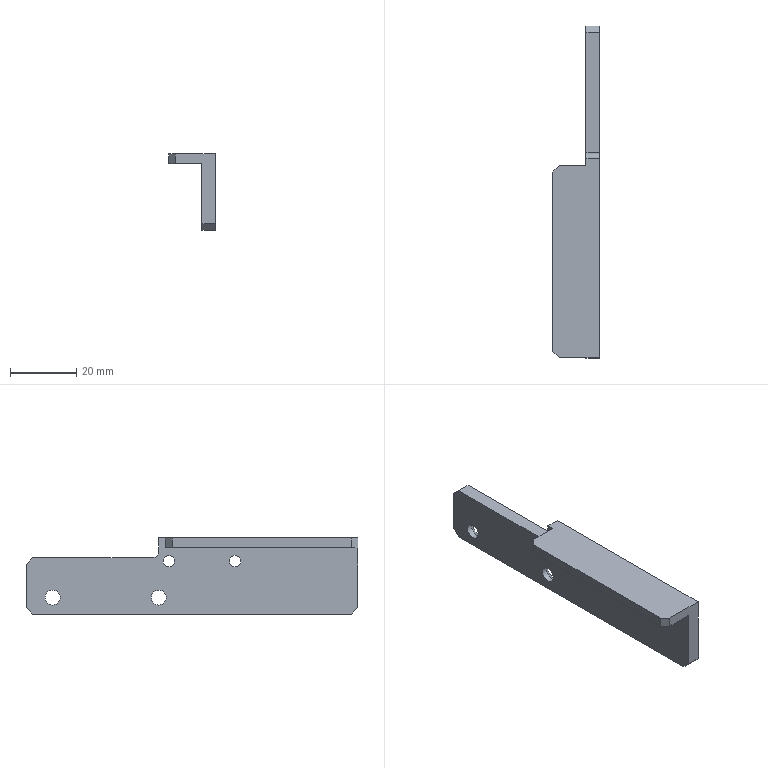Part | NX | features BREP 1 | 1 solid | 25 faces | box 14 x 100 x 23 mm | volume 9598 mm3 | plane 16 | cylinder 5 | cone 4 | commonest cylinder face diameters 3.4 x2 4.5 x2 4 x1
STEP:
#1=CARTESIAN_POINT('',(7.,50.,3.5));
#2=VERTEX_POINT('',#1);
#3=CARTESIAN_POINT('',(7.,50.,-9.5));
#4=VERTEX_POINT('',#3);
#5=CARTESIAN_POINT('',(7.,50.,11.5));
#6=DIRECTION('',(0.,0.,-1.));
#7=VECTOR('',#6,1000.);
#8=LINE('',#5,#7);
#9=EDGE_CURVE('',#2,#4,#8,.T.);
#10=ORIENTED_EDGE('',*,*,#9,.T.);
#11=CARTESIAN_POINT('',(3.,50.,-9.5));
#12=VERTEX_POINT('',#11);
#13=CARTESIAN_POINT('',(3.,50.,-9.5));
#14=DIRECTION('',(-1.,0.,0.));
#15=VECTOR('',#14,1000.);
#16=LINE('',#13,#15);
#17=EDGE_CURVE('',#4,#12,#16,.T.);
#18=ORIENTED_EDGE('',*,*,#17,.T.);
#19=CARTESIAN_POINT('',(3.,50.,3.5));
#20=VERTEX_POINT('',#19);
#21=CARTESIAN_POINT('',(3.,50.,-11.5));
#22=DIRECTION('',(0.,0.,-1.));
#23=VECTOR('',#22,1000.);
#24=LINE('',#21,#23);
#25=EDGE_CURVE('',#20,#12,#24,.T.);
#26=ORIENTED_EDGE('',*,*,#25,.F.);
#27=CARTESIAN_POINT('',(7.,50.,3.5));
#28=DIRECTION('',(1.,0.,0.));
#29=VECTOR('',#28,1000.);
#30=LINE('',#27,#29);
#31=EDGE_CURVE('',#20,#2,#30,.T.);
#32=ORIENTED_EDGE('',*,*,#31,.T.);
#33=EDGE_LOOP('',(#10,#18,#26,#32));
#34=FACE_BOUND('',#33,.T.);
#35=CARTESIAN_POINT('',(-7.,50.,11.5));
#36=DIRECTION('',(0.,-1.,0.));
#37=DIRECTION('',(0.,0.,1.));
#38=AXIS2_PLACEMENT_3D('',#35,#36,#37);
#39=PLANE('',#38);
#40=ADVANCED_FACE('',(#34),#39,.F.);
#41=CARTESIAN_POINT('',(7.,7.,1.03));
#42=VERTEX_POINT('',#41);
#43=CARTESIAN_POINT('',(7.,7.,4.5));
#44=DIRECTION('',(1.,0.,0.));
#45=DIRECTION('',(0.,0.,-1.));
#46=AXIS2_PLACEMENT_3D('',#43,#44,#45);
#47=CIRCLE('',#46,3.47);
#48=EDGE_CURVE('',#42,#42,#47,.T.);
#49=ORIENTED_EDGE('',*,*,#48,.F.);
#50=EDGE_LOOP('',(#49));
#51=FACE_BOUND('',#50,.T.);
#52=CARTESIAN_POINT('',(7.,-13.,1.03));
#53=VERTEX_POINT('',#52);
#54=CARTESIAN_POINT('',(7.,-13.,4.5));
#55=DIRECTION('',(1.,0.,0.));
#56=DIRECTION('',(0.,0.,-1.));
#57=AXIS2_PLACEMENT_3D('',#54,#55,#56);
#58=CIRCLE('',#57,3.47);
#59=EDGE_CURVE('',#53,#53,#58,.T.);
#60=ORIENTED_EDGE('',*,*,#59,.F.);
#61=EDGE_LOOP('',(#60));
#62=FACE_BOUND('',#61,.T.);
#63=CARTESIAN_POINT('',(7.,42.,-11.09));
#64=VERTEX_POINT('',#63);
#65=CARTESIAN_POINT('',(7.,42.,-6.5));
#66=DIRECTION('',(1.,0.,0.));
#67=DIRECTION('',(0.,0.,-1.));
#68=AXIS2_PLACEMENT_3D('',#65,#66,#67);
#69=CIRCLE('',#68,4.59);
#70=EDGE_CURVE('',#64,#64,#69,.T.);
#71=ORIENTED_EDGE('',*,*,#70,.F.);
#72=EDGE_LOOP('',(#71));
#73=FACE_BOUND('',#72,.T.);
#74=CARTESIAN_POINT('',(7.,10.,-11.09));
#75=VERTEX_POINT('',#74);
#76=CARTESIAN_POINT('',(7.,10.,-6.5));
#77=DIRECTION('',(1.,0.,0.));
#78=DIRECTION('',(0.,0.,-1.));
#79=AXIS2_PLACEMENT_3D('',#76,#77,#78);
#80=CIRCLE('',#79,4.59);
#81=EDGE_CURVE('',#75,#75,#80,.T.);
#82=ORIENTED_EDGE('',*,*,#81,.F.);
#83=EDGE_LOOP('',(#82));
#84=FACE_BOUND('',#83,.T.);
#85=CARTESIAN_POINT('',(7.,-50.,11.5));
#86=VERTEX_POINT('',#85);
#87=CARTESIAN_POINT('',(7.,-50.,-9.5));
#88=VERTEX_POINT('',#87);
#89=CARTESIAN_POINT('',(7.,-50.,11.5));
#90=DIRECTION('',(0.,0.,-1.));
#91=VECTOR('',#90,1000.);
#92=LINE('',#89,#91);
#93=EDGE_CURVE('',#86,#88,#92,.T.);
#94=ORIENTED_EDGE('',*,*,#93,.T.);
#95=CARTESIAN_POINT('',(7.,-48.,-11.5));
#96=VERTEX_POINT('',#95);
#97=CARTESIAN_POINT('',(7.,-50.,-9.5));
#98=DIRECTION('',(0.,0.7071,-0.7071));
#99=VECTOR('',#98,1000.);
#100=LINE('',#97,#99);
#101=EDGE_CURVE('',#88,#96,#100,.T.);
#102=ORIENTED_EDGE('',*,*,#101,.T.);
#103=CARTESIAN_POINT('',(7.,48.,-11.5));
#104=VERTEX_POINT('',#103);
#105=CARTESIAN_POINT('',(7.,-50.,-11.5));
#106=DIRECTION('',(0.,1.,0.));
#107=VECTOR('',#106,1000.);
#108=LINE('',#105,#107);
#109=EDGE_CURVE('',#96,#104,#108,.T.);
#110=ORIENTED_EDGE('',*,*,#109,.T.);
#111=CARTESIAN_POINT('',(7.,50.,-9.5));
#112=DIRECTION('',(0.,0.7071,0.7071));
#113=VECTOR('',#112,1000.);
#114=LINE('',#111,#113);
#115=EDGE_CURVE('',#104,#4,#114,.T.);
#116=ORIENTED_EDGE('',*,*,#115,.T.);
#117=ORIENTED_EDGE('',*,*,#9,.F.);
#118=CARTESIAN_POINT('',(7.,48.,5.5));
#119=VERTEX_POINT('',#118);
#120=CARTESIAN_POINT('',(7.,48.,5.5));
#121=DIRECTION('',(0.,-0.7071,0.7071));
#122=VECTOR('',#121,1000.);
#123=LINE('',#120,#122);
#124=EDGE_CURVE('',#2,#119,#123,.T.);
#125=ORIENTED_EDGE('',*,*,#124,.T.);
#126=CARTESIAN_POINT('',(7.,12.,5.5));
#127=VERTEX_POINT('',#126);
#128=CARTESIAN_POINT('',(7.,50.,5.5));
#129=DIRECTION('',(0.,1.,0.));
#130=VECTOR('',#129,1000.);
#131=LINE('',#128,#130);
#132=EDGE_CURVE('',#127,#119,#131,.T.);
#133=ORIENTED_EDGE('',*,*,#132,.F.);
#134=CARTESIAN_POINT('',(7.,10.,7.5));
#135=VERTEX_POINT('',#134);
#136=CARTESIAN_POINT('',(7.,12.,7.5));
#137=DIRECTION('',(-1.,0.,0.));
#138=DIRECTION('',(0.,0.,1.));
#139=AXIS2_PLACEMENT_3D('',#136,#137,#138);
#140=CIRCLE('',#139,2.);
#141=EDGE_CURVE('',#127,#135,#140,.T.);
#142=ORIENTED_EDGE('',*,*,#141,.T.);
#143=CARTESIAN_POINT('',(7.,10.,11.5));
#144=VERTEX_POINT('',#143);
#145=CARTESIAN_POINT('',(7.,10.,5.5));
#146=DIRECTION('',(0.,0.,1.));
#147=VECTOR('',#146,1000.);
#148=LINE('',#145,#147);
#149=EDGE_CURVE('',#135,#144,#148,.T.);
#150=ORIENTED_EDGE('',*,*,#149,.T.);
#151=CARTESIAN_POINT('',(7.,-50.,11.5));
#152=DIRECTION('',(0.,1.,0.));
#153=VECTOR('',#152,1000.);
#154=LINE('',#151,#153);
#155=EDGE_CURVE('',#86,#144,#154,.T.);
#156=ORIENTED_EDGE('',*,*,#155,.F.);
#157=EDGE_LOOP('',(#94,#102,#110,#116,#117,#125,#133,#142,#150,#156));
#158=FACE_BOUND('',#157,.T.);
#159=CARTESIAN_POINT('',(7.,-50.,11.5));
#160=DIRECTION('',(-1.,0.,0.));
#161=DIRECTION('',(0.,0.,-1.));
#162=AXIS2_PLACEMENT_3D('',#159,#160,#161);
#163=PLANE('',#162);
#164=ADVANCED_FACE('',(#51,#62,#73,#84,#158),#163,.F.);
#165=CARTESIAN_POINT('',(-7.,-48.,8.5));
#166=VERTEX_POINT('',#165);
#167=CARTESIAN_POINT('',(-7.,6.,8.5));
#168=VERTEX_POINT('',#167);
#169=CARTESIAN_POINT('',(-7.,-72.361,8.5));
#170=DIRECTION('',(0.,1.,0.));
#171=VECTOR('',#170,1000.);
#172=LINE('',#169,#171);
#173=EDGE_CURVE('',#166,#168,#172,.T.);
#174=ORIENTED_EDGE('',*,*,#173,.F.);
#175=CARTESIAN_POINT('',(-7.,-48.,11.5));
#176=VERTEX_POINT('',#175);
#177=CARTESIAN_POINT('',(-7.,-48.,11.5));
#178=DIRECTION('',(0.,0.,1.));
#179=VECTOR('',#178,1000.);
#180=LINE('',#177,#179);
#181=EDGE_CURVE('',#166,#176,#180,.T.);
#182=ORIENTED_EDGE('',*,*,#181,.T.);
#183=CARTESIAN_POINT('',(-7.,6.,11.5));
#184=VERTEX_POINT('',#183);
#185=CARTESIAN_POINT('',(-7.,-50.,11.5));
#186=DIRECTION('',(0.,-1.,0.));
#187=VECTOR('',#186,1000.);
#188=LINE('',#185,#187);
#189=EDGE_CURVE('',#184,#176,#188,.T.);
#190=ORIENTED_EDGE('',*,*,#189,.F.);
#191=CARTESIAN_POINT('',(-7.,6.,11.5));
#192=DIRECTION('',(0.,0.,-1.));
#193=VECTOR('',#192,1000.);
#194=LINE('',#191,#193);
#195=EDGE_CURVE('',#184,#168,#194,.T.);
#196=ORIENTED_EDGE('',*,*,#195,.T.);
#197=EDGE_LOOP('',(#174,#182,#190,#196));
#198=FACE_BOUND('',#197,.T.);
#199=CARTESIAN_POINT('',(-7.,-50.,11.5));
#200=DIRECTION('',(1.,0.,0.));
#201=DIRECTION('',(0.,0.,1.));
#202=AXIS2_PLACEMENT_3D('',#199,#200,#201);
#203=PLANE('',#202);
#204=ADVANCED_FACE('',(#198),#203,.F.);
#205=CARTESIAN_POINT('',(3.,-50.,-9.5));
#206=VERTEX_POINT('',#205);
#207=CARTESIAN_POINT('',(3.,-50.,8.5));
#208=VERTEX_POINT('',#207);
#209=CARTESIAN_POINT('',(3.,-50.,-11.5));
#210=DIRECTION('',(0.,0.,1.));
#211=VECTOR('',#210,1000.);
#212=LINE('',#209,#211);
#213=EDGE_CURVE('',#206,#208,#212,.T.);
#214=ORIENTED_EDGE('',*,*,#213,.F.);
#215=CARTESIAN_POINT('',(7.,-50.,-9.5));
#216=DIRECTION('',(1.,0.,0.));
#217=VECTOR('',#216,1000.);
#218=LINE('',#215,#217);
#219=EDGE_CURVE('',#206,#88,#218,.T.);
#220=ORIENTED_EDGE('',*,*,#219,.T.);
#221=ORIENTED_EDGE('',*,*,#93,.F.);
#222=CARTESIAN_POINT('',(-5.,-50.,11.5));
#223=VERTEX_POINT('',#222);
#224=CARTESIAN_POINT('',(-7.,-50.,11.5));
#225=DIRECTION('',(1.,0.,0.));
#226=VECTOR('',#225,1000.);
#227=LINE('',#224,#226);
#228=EDGE_CURVE('',#223,#86,#227,.T.);
#229=ORIENTED_EDGE('',*,*,#228,.F.);
#230=CARTESIAN_POINT('',(-5.,-50.,8.5));
#231=VERTEX_POINT('',#230);
#232=CARTESIAN_POINT('',(-5.,-50.,11.5));
#233=DIRECTION('',(0.,0.,-1.));
#234=VECTOR('',#233,1000.);
#235=LINE('',#232,#234);
#236=EDGE_CURVE('',#223,#231,#235,.T.);
#237=ORIENTED_EDGE('',*,*,#236,.T.);
#238=CARTESIAN_POINT('',(-7.,-50.,8.5));
#239=DIRECTION('',(-1.,0.,0.));
#240=VECTOR('',#239,1000.);
#241=LINE('',#238,#240);
#242=EDGE_CURVE('',#208,#231,#241,.T.);
#243=ORIENTED_EDGE('',*,*,#242,.F.);
#244=EDGE_LOOP('',(#214,#220,#221,#229,#237,#243));
#245=FACE_BOUND('',#244,.T.);
#246=CARTESIAN_POINT('',(-7.,-50.,11.5));
#247=DIRECTION('',(0.,1.,0.));
#248=DIRECTION('',(0.,0.,-1.));
#249=AXIS2_PLACEMENT_3D('',#246,#247,#248);
#250=PLANE('',#249);
#251=ADVANCED_FACE('',(#245),#250,.F.);
#252=ORIENTED_EDGE('',*,*,#189,.T.);
#253=CARTESIAN_POINT('',(-5.,-50.,11.5));
#254=DIRECTION('',(0.7071,-0.7071,0.));
#255=VECTOR('',#254,1000.);
#256=LINE('',#253,#255);
#257=EDGE_CURVE('',#176,#223,#256,.T.);
#258=ORIENTED_EDGE('',*,*,#257,.T.);
#259=ORIENTED_EDGE('',*,*,#228,.T.);
#260=ORIENTED_EDGE('',*,*,#155,.T.);
#261=CARTESIAN_POINT('',(3.,10.,11.5));
#262=VERTEX_POINT('',#261);
#263=CARTESIAN_POINT('',(-7.,10.,11.5));
#264=DIRECTION('',(1.,0.,0.));
#265=VECTOR('',#264,1000.);
#266=LINE('',#263,#265);
#267=EDGE_CURVE('',#262,#144,#266,.T.);
#268=ORIENTED_EDGE('',*,*,#267,.F.);
#269=CARTESIAN_POINT('',(3.,8.,11.5));
#270=VERTEX_POINT('',#269);
#271=CARTESIAN_POINT('',(3.,8.,11.5));
#272=DIRECTION('',(0.,1.,0.));
#273=VECTOR('',#272,1000.);
#274=LINE('',#271,#273);
#275=EDGE_CURVE('',#270,#262,#274,.T.);
#276=ORIENTED_EDGE('',*,*,#275,.F.);
#277=CARTESIAN_POINT('',(-5.,8.,11.5));
#278=VERTEX_POINT('',#277);
#279=CARTESIAN_POINT('',(3.,8.,11.5));
#280=DIRECTION('',(1.,0.,0.));
#281=VECTOR('',#280,1000.);
#282=LINE('',#279,#281);
#283=EDGE_CURVE('',#278,#270,#282,.T.);
#284=ORIENTED_EDGE('',*,*,#283,.F.);
#285=CARTESIAN_POINT('',(-5.,8.,11.5));
#286=DIRECTION('',(-0.7071,-0.7071,0.));
#287=VECTOR('',#286,1000.);
#288=LINE('',#285,#287);
#289=EDGE_CURVE('',#278,#184,#288,.T.);
#290=ORIENTED_EDGE('',*,*,#289,.T.);
#291=EDGE_LOOP('',(#252,#258,#259,#260,#268,#276,#284,#290));
#292=FACE_BOUND('',#291,.T.);
#293=CARTESIAN_POINT('',(0.,0.,11.5));
#294=DIRECTION('',(0.,0.,-1.));
#295=DIRECTION('',(1.,0.,0.));
#296=AXIS2_PLACEMENT_3D('',#293,#294,#295);
#297=PLANE('',#296);
#298=ADVANCED_FACE('',(#292),#297,.F.);
#299=ORIENTED_EDGE('',*,*,#109,.F.);
#300=CARTESIAN_POINT('',(3.,-48.,-11.5));
#301=VERTEX_POINT('',#300);
#302=CARTESIAN_POINT('',(3.,-48.,-11.5));
#303=DIRECTION('',(-1.,0.,0.));
#304=VECTOR('',#303,1000.);
#305=LINE('',#302,#304);
#306=EDGE_CURVE('',#96,#301,#305,.T.);
#307=ORIENTED_EDGE('',*,*,#306,.T.);
#308=CARTESIAN_POINT('',(3.,48.,-11.5));
#309=VERTEX_POINT('',#308);
#310=CARTESIAN_POINT('',(3.,-72.361,-11.5));
#311=DIRECTION('',(0.,1.,0.));
#312=VECTOR('',#311,1000.);
#313=LINE('',#310,#312);
#314=EDGE_CURVE('',#301,#309,#313,.T.);
#315=ORIENTED_EDGE('',*,*,#314,.T.);
#316=CARTESIAN_POINT('',(7.,48.,-11.5));
#317=DIRECTION('',(1.,0.,0.));
#318=VECTOR('',#317,1000.);
#319=LINE('',#316,#318);
#320=EDGE_CURVE('',#309,#104,#319,.T.);
#321=ORIENTED_EDGE('',*,*,#320,.T.);
#322=EDGE_LOOP('',(#299,#307,#315,#321));
#323=FACE_BOUND('',#322,.T.);
#324=CARTESIAN_POINT('',(0.,0.,-11.5));
#325=DIRECTION('',(0.,0.,-1.));
#326=DIRECTION('',(1.,0.,0.));
#327=AXIS2_PLACEMENT_3D('',#324,#325,#326);
#328=PLANE('',#327);
#329=ADVANCED_FACE('',(#323),#328,.T.);
#330=CARTESIAN_POINT('',(3.,7.,2.8));
#331=VERTEX_POINT('',#330);
#332=CARTESIAN_POINT('',(3.,7.,4.5));
#333=DIRECTION('',(1.,0.,0.));
#334=DIRECTION('',(0.,0.,-1.));
#335=AXIS2_PLACEMENT_3D('',#332,#333,#334);
#336=CIRCLE('',#335,1.7);
#337=EDGE_CURVE('',#331,#331,#336,.T.);
#338=ORIENTED_EDGE('',*,*,#337,.T.);
#339=EDGE_LOOP('',(#338));
#340=FACE_BOUND('',#339,.T.);
#341=CARTESIAN_POINT('',(3.,-13.,2.8));
#342=VERTEX_POINT('',#341);
#343=CARTESIAN_POINT('',(3.,-13.,4.5));
#344=DIRECTION('',(1.,0.,0.));
#345=DIRECTION('',(0.,0.,-1.));
#346=AXIS2_PLACEMENT_3D('',#343,#344,#345);
#347=CIRCLE('',#346,1.7);
#348=EDGE_CURVE('',#342,#342,#347,.T.);
#349=ORIENTED_EDGE('',*,*,#348,.T.);
#350=EDGE_LOOP('',(#349));
#351=FACE_BOUND('',#350,.T.);
#352=CARTESIAN_POINT('',(3.,42.,-8.75));
#353=VERTEX_POINT('',#352);
#354=CARTESIAN_POINT('',(3.,42.,-6.5));
#355=DIRECTION('',(1.,0.,0.));
#356=DIRECTION('',(0.,0.,-1.));
#357=AXIS2_PLACEMENT_3D('',#354,#355,#356);
#358=CIRCLE('',#357,2.25);
#359=EDGE_CURVE('',#353,#353,#358,.T.);
#360=ORIENTED_EDGE('',*,*,#359,.T.);
#361=EDGE_LOOP('',(#360));
#362=FACE_BOUND('',#361,.T.);
#363=CARTESIAN_POINT('',(3.,10.,-8.75));
#364=VERTEX_POINT('',#363);
#365=CARTESIAN_POINT('',(3.,10.,-6.5));
#366=DIRECTION('',(1.,0.,0.));
#367=DIRECTION('',(0.,0.,-1.));
#368=AXIS2_PLACEMENT_3D('',#365,#366,#367);
#369=CIRCLE('',#368,2.25);
#370=EDGE_CURVE('',#364,#364,#369,.T.);
#371=ORIENTED_EDGE('',*,*,#370,.T.);
#372=EDGE_LOOP('',(#371));
#373=FACE_BOUND('',#372,.T.);
#374=ORIENTED_EDGE('',*,*,#314,.F.);
#375=CARTESIAN_POINT('',(3.,-50.,-9.5));
#376=DIRECTION('',(0.,-0.7071,0.7071));
#377=VECTOR('',#376,1000.);
#378=LINE('',#375,#377);
#379=EDGE_CURVE('',#301,#206,#378,.T.);
#380=ORIENTED_EDGE('',*,*,#379,.T.);
#381=ORIENTED_EDGE('',*,*,#213,.T.);
#382=CARTESIAN_POINT('',(3.,8.,8.5));
#383=VERTEX_POINT('',#382);
#384=CARTESIAN_POINT('',(3.,-72.361,8.5));
#385=DIRECTION('',(0.,1.,0.));
#386=VECTOR('',#385,1000.);
#387=LINE('',#384,#386);
#388=EDGE_CURVE('',#208,#383,#387,.T.);
#389=ORIENTED_EDGE('',*,*,#388,.T.);
#390=CARTESIAN_POINT('',(3.,8.,8.5));
#391=DIRECTION('',(0.,0.,-1.));
#392=VECTOR('',#391,1000.);
#393=LINE('',#390,#392);
#394=EDGE_CURVE('',#270,#383,#393,.T.);
#395=ORIENTED_EDGE('',*,*,#394,.F.);
#396=ORIENTED_EDGE('',*,*,#275,.T.);
#397=CARTESIAN_POINT('',(3.,10.,7.5));
#398=VERTEX_POINT('',#397);
#399=CARTESIAN_POINT('',(3.,10.,-11.5));
#400=DIRECTION('',(0.,0.,-1.));
#401=VECTOR('',#400,1000.);
#402=LINE('',#399,#401);
#403=EDGE_CURVE('',#262,#398,#402,.T.);
#404=ORIENTED_EDGE('',*,*,#403,.T.);
#405=CARTESIAN_POINT('',(3.,12.,5.5));
#406=VERTEX_POINT('',#405);
#407=CARTESIAN_POINT('',(3.,12.,7.5));
#408=DIRECTION('',(1.,0.,0.));
#409=DIRECTION('',(0.,0.,-1.));
#410=AXIS2_PLACEMENT_3D('',#407,#408,#409);
#411=CIRCLE('',#410,2.);
#412=EDGE_CURVE('',#398,#406,#411,.T.);
#413=ORIENTED_EDGE('',*,*,#412,.T.);
#414=CARTESIAN_POINT('',(3.,48.,5.5));
#415=VERTEX_POINT('',#414);
#416=CARTESIAN_POINT('',(3.,-72.361,5.5));
#417=DIRECTION('',(0.,-1.,0.));
#418=VECTOR('',#417,1000.);
#419=LINE('',#416,#418);
#420=EDGE_CURVE('',#415,#406,#419,.T.);
#421=ORIENTED_EDGE('',*,*,#420,.F.);
#422=CARTESIAN_POINT('',(3.,48.,5.5));
#423=DIRECTION('',(0.,0.7071,-0.7071));
#424=VECTOR('',#423,1000.);
#425=LINE('',#422,#424);
#426=EDGE_CURVE('',#415,#20,#425,.T.);
#427=ORIENTED_EDGE('',*,*,#426,.T.);
#428=ORIENTED_EDGE('',*,*,#25,.T.);
#429=CARTESIAN_POINT('',(3.,50.,-9.5));
#430=DIRECTION('',(0.,-0.7071,-0.7071));
#431=VECTOR('',#430,1000.);
#432=LINE('',#429,#431);
#433=EDGE_CURVE('',#12,#309,#432,.T.);
#434=ORIENTED_EDGE('',*,*,#433,.T.);
#435=EDGE_LOOP('',(#374,#380,#381,#389,#395,#396,#404,#413,#421,#427,#428,#434));
#436=FACE_BOUND('',#435,.T.);
#437=CARTESIAN_POINT('',(3.,-72.361,-11.5));
#438=DIRECTION('',(1.,0.,0.));
#439=DIRECTION('',(0.,0.,1.));
#440=AXIS2_PLACEMENT_3D('',#437,#438,#439);
#441=PLANE('',#440);
#442=ADVANCED_FACE('',(#340,#351,#362,#373,#436),#441,.F.);
#443=ORIENTED_EDGE('',*,*,#242,.T.);
#444=CARTESIAN_POINT('',(-5.,-50.,8.5));
#445=DIRECTION('',(-0.7071,0.7071,0.));
#446=VECTOR('',#445,1000.);
#447=LINE('',#444,#446);
#448=EDGE_CURVE('',#231,#166,#447,.T.);
#449=ORIENTED_EDGE('',*,*,#448,.T.);
#450=ORIENTED_EDGE('',*,*,#173,.T.);
#451=CARTESIAN_POINT('',(-5.,8.,8.5));
#452=VERTEX_POINT('',#451);
#453=CARTESIAN_POINT('',(-5.,8.,8.5));
#454=DIRECTION('',(0.7071,0.7071,0.));
#455=VECTOR('',#454,1000.);
#456=LINE('',#453,#455);
#457=EDGE_CURVE('',#168,#452,#456,.T.);
#458=ORIENTED_EDGE('',*,*,#457,.T.);
#459=CARTESIAN_POINT('',(3.,8.,8.5));
#460=DIRECTION('',(-1.,0.,0.));
#461=VECTOR('',#460,1000.);
#462=LINE('',#459,#461);
#463=EDGE_CURVE('',#383,#452,#462,.T.);
#464=ORIENTED_EDGE('',*,*,#463,.F.);
#465=ORIENTED_EDGE('',*,*,#388,.F.);
#466=EDGE_LOOP('',(#443,#449,#450,#458,#464,#465));
#467=FACE_BOUND('',#466,.T.);
#468=CARTESIAN_POINT('',(-7.,-72.361,8.5));
#469=DIRECTION('',(0.,0.,1.));
#470=DIRECTION('',(-1.,0.,0.));
#471=AXIS2_PLACEMENT_3D('',#468,#469,#470);
#472=PLANE('',#471);
#473=ADVANCED_FACE('',(#467),#472,.F.);
#474=ORIENTED_EDGE('',*,*,#132,.T.);
#475=CARTESIAN_POINT('',(3.,48.,5.5));
#476=DIRECTION('',(-1.,0.,0.));
#477=VECTOR('',#476,1000.);
#478=LINE('',#475,#477);
#479=EDGE_CURVE('',#119,#415,#478,.T.);
#480=ORIENTED_EDGE('',*,*,#479,.T.);
#481=ORIENTED_EDGE('',*,*,#420,.T.);
#482=CARTESIAN_POINT('',(0.,12.,5.5));
#483=DIRECTION('',(1.,0.,0.));
#484=VECTOR('',#483,1000.);
#485=LINE('',#482,#484);
#486=EDGE_CURVE('',#406,#127,#485,.T.);
#487=ORIENTED_EDGE('',*,*,#486,.T.);
#488=EDGE_LOOP('',(#474,#480,#481,#487));
#489=FACE_BOUND('',#488,.T.);
#490=CARTESIAN_POINT('',(0.,0.,5.5));
#491=DIRECTION('',(0.,0.,1.));
#492=DIRECTION('',(-1.,0.,0.));
#493=AXIS2_PLACEMENT_3D('',#490,#491,#492);
#494=PLANE('',#493);
#495=ADVANCED_FACE('',(#489),#494,.T.);
#496=ORIENTED_EDGE('',*,*,#403,.F.);
#497=ORIENTED_EDGE('',*,*,#267,.T.);
#498=ORIENTED_EDGE('',*,*,#149,.F.);
#499=CARTESIAN_POINT('',(-7.,10.,7.5));
#500=DIRECTION('',(-1.,0.,0.));
#501=VECTOR('',#500,1000.);
#502=LINE('',#499,#501);
#503=EDGE_CURVE('',#135,#398,#502,.T.);
#504=ORIENTED_EDGE('',*,*,#503,.T.);
#505=EDGE_LOOP('',(#496,#497,#498,#504));
#506=FACE_BOUND('',#505,.T.);
#507=CARTESIAN_POINT('',(-7.,10.,5.5));
#508=DIRECTION('',(0.,-1.,0.));
#509=DIRECTION('',(0.,0.,1.));
#510=AXIS2_PLACEMENT_3D('',#507,#508,#509);
#511=PLANE('',#510);
#512=ADVANCED_FACE('',(#506),#511,.F.);
#513=CARTESIAN_POINT('',(4.66,10.,-8.75));
#514=VERTEX_POINT('',#513);
#515=CARTESIAN_POINT('',(4.66,10.,-6.5));
#516=DIRECTION('',(1.,0.,0.));
#517=DIRECTION('',(0.,0.,-1.));
#518=AXIS2_PLACEMENT_3D('',#515,#516,#517);
#519=CIRCLE('',#518,2.25);
#520=EDGE_CURVE('',#514,#514,#519,.T.);
#521=ORIENTED_EDGE('',*,*,#520,.T.);
#522=EDGE_LOOP('',(#521));
#523=FACE_BOUND('',#522,.T.);
#524=ORIENTED_EDGE('',*,*,#370,.F.);
#525=EDGE_LOOP('',(#524));
#526=FACE_BOUND('',#525,.T.);
#527=CARTESIAN_POINT('',(7.,10.,-6.5));
#528=DIRECTION('',(1.,0.,0.));
#529=DIRECTION('',(0.,0.,1.));
#530=AXIS2_PLACEMENT_3D('',#527,#528,#529);
#531=CYLINDRICAL_SURFACE('',#530,2.25);
#532=ADVANCED_FACE('',(#523,#526),#531,.F.);
#533=ORIENTED_EDGE('',*,*,#520,.F.);
#534=EDGE_LOOP('',(#533));
#535=FACE_BOUND('',#534,.T.);
#536=ORIENTED_EDGE('',*,*,#81,.T.);
#537=EDGE_LOOP('',(#536));
#538=FACE_BOUND('',#537,.T.);
#539=CARTESIAN_POINT('',(7.,10.,-6.5));
#540=DIRECTION('',(1.,0.,0.));
#541=DIRECTION('',(0.,0.,1.));
#542=AXIS2_PLACEMENT_3D('',#539,#540,#541);
#543=CONICAL_SURFACE('',#542,4.59,0.7854);
#544=ADVANCED_FACE('',(#535,#538),#543,.F.);
#545=CARTESIAN_POINT('',(4.66,42.,-8.75));
#546=VERTEX_POINT('',#545);
#547=CARTESIAN_POINT('',(4.66,42.,-6.5));
#548=DIRECTION('',(1.,0.,0.));
#549=DIRECTION('',(0.,0.,-1.));
#550=AXIS2_PLACEMENT_3D('',#547,#548,#549);
#551=CIRCLE('',#550,2.25);
#552=EDGE_CURVE('',#546,#546,#551,.T.);
#553=ORIENTED_EDGE('',*,*,#552,.T.);
#554=EDGE_LOOP('',(#553));
#555=FACE_BOUND('',#554,.T.);
#556=ORIENTED_EDGE('',*,*,#359,.F.);
#557=EDGE_LOOP('',(#556));
#558=FACE_BOUND('',#557,.T.);
#559=CARTESIAN_POINT('',(7.,42.,-6.5));
#560=DIRECTION('',(1.,0.,0.));
#561=DIRECTION('',(0.,0.,1.));
#562=AXIS2_PLACEMENT_3D('',#559,#560,#561);
#563=CYLINDRICAL_SURFACE('',#562,2.25);
#564=ADVANCED_FACE('',(#555,#558),#563,.F.);
#565=ORIENTED_EDGE('',*,*,#552,.F.);
#566=EDGE_LOOP('',(#565));
#567=FACE_BOUND('',#566,.T.);
#568=ORIENTED_EDGE('',*,*,#70,.T.);
#569=EDGE_LOOP('',(#568));
#570=FACE_BOUND('',#569,.T.);
#571=CARTESIAN_POINT('',(7.,42.,-6.5));
#572=DIRECTION('',(1.,0.,0.));
#573=DIRECTION('',(0.,0.,1.));
#574=AXIS2_PLACEMENT_3D('',#571,#572,#573);
#575=CONICAL_SURFACE('',#574,4.59,0.7854);
#576=ADVANCED_FACE('',(#567,#570),#575,.F.);
#577=ORIENTED_EDGE('',*,*,#412,.F.);
#578=ORIENTED_EDGE('',*,*,#503,.F.);
#579=ORIENTED_EDGE('',*,*,#141,.F.);
#580=ORIENTED_EDGE('',*,*,#486,.F.);
#581=EDGE_LOOP('',(#577,#578,#579,#580));
#582=FACE_BOUND('',#581,.T.);
#583=CARTESIAN_POINT('',(0.,12.,7.5));
#584=DIRECTION('',(1.,0.,0.));
#585=DIRECTION('',(0.,0.,1.));
#586=AXIS2_PLACEMENT_3D('',#583,#584,#585);
#587=CYLINDRICAL_SURFACE('',#586,2.);
#588=ADVANCED_FACE('',(#582),#587,.F.);
#589=CARTESIAN_POINT('',(5.23,-13.,2.8));
#590=VERTEX_POINT('',#589);
#591=CARTESIAN_POINT('',(5.23,-13.,4.5));
#592=DIRECTION('',(1.,0.,0.));
#593=DIRECTION('',(0.,0.,-1.));
#594=AXIS2_PLACEMENT_3D('',#591,#592,#593);
#595=CIRCLE('',#594,1.7);
#596=EDGE_CURVE('',#590,#590,#595,.T.);
#597=ORIENTED_EDGE('',*,*,#596,.T.);
#598=EDGE_LOOP('',(#597));
#599=FACE_BOUND('',#598,.T.);
#600=ORIENTED_EDGE('',*,*,#348,.F.);
#601=EDGE_LOOP('',(#600));
#602=FACE_BOUND('',#601,.T.);
#603=CARTESIAN_POINT('',(7.,-13.,4.5));
#604=DIRECTION('',(1.,0.,0.));
#605=DIRECTION('',(0.,0.,1.));
#606=AXIS2_PLACEMENT_3D('',#603,#604,#605);
#607=CYLINDRICAL_SURFACE('',#606,1.7);
#608=ADVANCED_FACE('',(#599,#602),#607,.F.);
#609=ORIENTED_EDGE('',*,*,#596,.F.);
#610=EDGE_LOOP('',(#609));
#611=FACE_BOUND('',#610,.T.);
#612=ORIENTED_EDGE('',*,*,#59,.T.);
#613=EDGE_LOOP('',(#612));
#614=FACE_BOUND('',#613,.T.);
#615=CARTESIAN_POINT('',(7.,-13.,4.5));
#616=DIRECTION('',(1.,0.,0.));
#617=DIRECTION('',(0.,0.,1.));
#618=AXIS2_PLACEMENT_3D('',#615,#616,#617);
#619=CONICAL_SURFACE('',#618,3.47,0.7854);
#620=ADVANCED_FACE('',(#611,#614),#619,.F.);
#621=CARTESIAN_POINT('',(5.23,7.,2.8));
#622=VERTEX_POINT('',#621);
#623=CARTESIAN_POINT('',(5.23,7.,4.5));
#624=DIRECTION('',(1.,0.,0.));
#625=DIRECTION('',(0.,0.,-1.));
#626=AXIS2_PLACEMENT_3D('',#623,#624,#625);
#627=CIRCLE('',#626,1.7);
#628=EDGE_CURVE('',#622,#622,#627,.T.);
#629=ORIENTED_EDGE('',*,*,#628,.T.);
#630=EDGE_LOOP('',(#629));
#631=FACE_BOUND('',#630,.T.);
#632=ORIENTED_EDGE('',*,*,#337,.F.);
#633=EDGE_LOOP('',(#632));
#634=FACE_BOUND('',#633,.T.);
#635=CARTESIAN_POINT('',(7.,7.,4.5));
#636=DIRECTION('',(1.,0.,0.));
#637=DIRECTION('',(0.,0.,1.));
#638=AXIS2_PLACEMENT_3D('',#635,#636,#637);
#639=CYLINDRICAL_SURFACE('',#638,1.7);
#640=ADVANCED_FACE('',(#631,#634),#639,.F.);
#641=ORIENTED_EDGE('',*,*,#628,.F.);
#642=EDGE_LOOP('',(#641));
#643=FACE_BOUND('',#642,.T.);
#644=ORIENTED_EDGE('',*,*,#48,.T.);
#645=EDGE_LOOP('',(#644));
#646=FACE_BOUND('',#645,.T.);
#647=CARTESIAN_POINT('',(7.,7.,4.5));
#648=DIRECTION('',(1.,0.,0.));
#649=DIRECTION('',(0.,0.,1.));
#650=AXIS2_PLACEMENT_3D('',#647,#648,#649);
#651=CONICAL_SURFACE('',#650,3.47,0.7854);
#652=ADVANCED_FACE('',(#643,#646),#651,.F.);
#653=ORIENTED_EDGE('',*,*,#463,.T.);
#654=CARTESIAN_POINT('',(-5.,8.,0.));
#655=DIRECTION('',(0.,0.,1.));
#656=VECTOR('',#655,1000.);
#657=LINE('',#654,#656);
#658=EDGE_CURVE('',#452,#278,#657,.T.);
#659=ORIENTED_EDGE('',*,*,#658,.T.);
#660=ORIENTED_EDGE('',*,*,#283,.T.);
#661=ORIENTED_EDGE('',*,*,#394,.T.);
#662=EDGE_LOOP('',(#653,#659,#660,#661));
#663=FACE_BOUND('',#662,.T.);
#664=CARTESIAN_POINT('',(0.,8.,0.));
#665=DIRECTION('',(0.,-1.,0.));
#666=DIRECTION('',(0.,0.,1.));
#667=AXIS2_PLACEMENT_3D('',#664,#665,#666);
#668=PLANE('',#667);
#669=ADVANCED_FACE('',(#663),#668,.F.);
#670=ORIENTED_EDGE('',*,*,#379,.F.);
#671=ORIENTED_EDGE('',*,*,#306,.F.);
#672=ORIENTED_EDGE('',*,*,#101,.F.);
#673=ORIENTED_EDGE('',*,*,#219,.F.);
#674=EDGE_LOOP('',(#670,#671,#672,#673));
#675=FACE_BOUND('',#674,.T.);
#676=CARTESIAN_POINT('',(-7.,-50.,-9.5));
#677=DIRECTION('',(0.,-0.7071,-0.7071));
#678=DIRECTION('',(1.,0.,0.));
#679=AXIS2_PLACEMENT_3D('',#676,#677,#678);
#680=PLANE('',#679);
#681=ADVANCED_FACE('',(#675),#680,.T.);
#682=ORIENTED_EDGE('',*,*,#257,.F.);
#683=ORIENTED_EDGE('',*,*,#181,.F.);
#684=ORIENTED_EDGE('',*,*,#448,.F.);
#685=ORIENTED_EDGE('',*,*,#236,.F.);
#686=EDGE_LOOP('',(#682,#683,#684,#685));
#687=FACE_BOUND('',#686,.T.);
#688=CARTESIAN_POINT('',(-5.,-50.,11.5));
#689=DIRECTION('',(0.7071,0.7071,0.));
#690=DIRECTION('',(0.,0.,1.));
#691=AXIS2_PLACEMENT_3D('',#688,#689,#690);
#692=PLANE('',#691);
#693=ADVANCED_FACE('',(#687),#692,.F.);
#694=ORIENTED_EDGE('',*,*,#457,.F.);
#695=ORIENTED_EDGE('',*,*,#195,.F.);
#696=ORIENTED_EDGE('',*,*,#289,.F.);
#697=ORIENTED_EDGE('',*,*,#658,.F.);
#698=EDGE_LOOP('',(#694,#695,#696,#697));
#699=FACE_BOUND('',#698,.T.);
#700=CARTESIAN_POINT('',(-5.,8.,0.));
#701=DIRECTION('',(0.7071,-0.7071,0.));
#702=DIRECTION('',(0.,0.,-1.));
#703=AXIS2_PLACEMENT_3D('',#700,#701,#702);
#704=PLANE('',#703);
#705=ADVANCED_FACE('',(#699),#704,.F.);
#706=ORIENTED_EDGE('',*,*,#115,.F.);
#707=ORIENTED_EDGE('',*,*,#320,.F.);
#708=ORIENTED_EDGE('',*,*,#433,.F.);
#709=ORIENTED_EDGE('',*,*,#17,.F.);
#710=EDGE_LOOP('',(#706,#707,#708,#709));
#711=FACE_BOUND('',#710,.T.);
#712=CARTESIAN_POINT('',(-7.,50.,-9.5));
#713=DIRECTION('',(0.,0.7071,-0.7071));
#714=DIRECTION('',(-1.,0.,0.));
#715=AXIS2_PLACEMENT_3D('',#712,#713,#714);
#716=PLANE('',#715);
#717=ADVANCED_FACE('',(#711),#716,.T.);
#718=ORIENTED_EDGE('',*,*,#124,.F.);
#719=ORIENTED_EDGE('',*,*,#31,.F.);
#720=ORIENTED_EDGE('',*,*,#426,.F.);
#721=ORIENTED_EDGE('',*,*,#479,.F.);
#722=EDGE_LOOP('',(#718,#719,#720,#721));
#723=FACE_BOUND('',#722,.T.);
#724=CARTESIAN_POINT('',(0.,48.,5.5));
#725=DIRECTION('',(0.,0.7071,0.7071));
#726=DIRECTION('',(-1.,0.,0.));
#727=AXIS2_PLACEMENT_3D('',#724,#725,#726);
#728=PLANE('',#727);
#729=ADVANCED_FACE('',(#723),#728,.T.);
#730=CLOSED_SHELL('',(#40,#164,#204,#251,#298,#329,#442,#473,#495,#512,#532,#544,#564,#576,#588,#608,#620,#640,#652,#669,#681,#693,#705,#717,#729));
#731=MANIFOLD_SOLID_BREP('',#730);
#732=(LENGTH_UNIT()NAMED_UNIT(*)SI_UNIT(.MILLI.,.METRE.));
#733=UNCERTAINTY_MEASURE_WITH_UNIT(LENGTH_MEASURE(0.00001),#732,'','');
#734=(NAMED_UNIT(*)PLANE_ANGLE_UNIT()SI_UNIT($,.RADIAN.));
#735=(NAMED_UNIT(*)SI_UNIT($,.STERADIAN.)SOLID_ANGLE_UNIT());
#736=(GEOMETRIC_REPRESENTATION_CONTEXT(3)GLOBAL_UNCERTAINTY_ASSIGNED_CONTEXT((#733))GLOBAL_UNIT_ASSIGNED_CONTEXT((#732,#734,#735))REPRESENTATION_CONTEXT('',''));
#737=ADVANCED_BREP_SHAPE_REPRESENTATION('',(#731),#736);